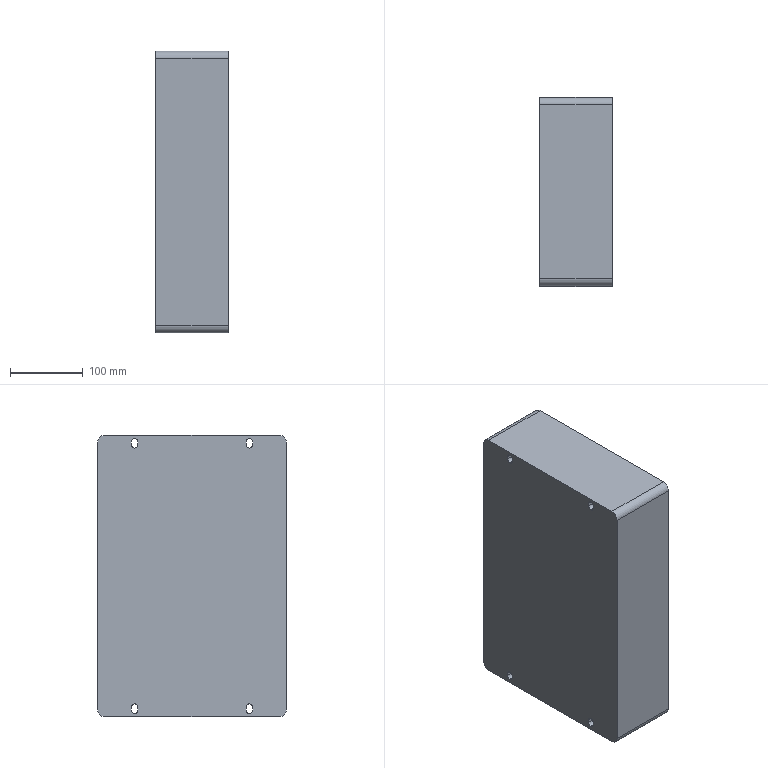Part | SolidWorks | 1 solid | 30 faces | box 100 x 260 x 388 mm | volume 10039569 mm3 | cylinder 16 | plane 14 | commonest cylinder face diameters 9 x12 20 x4
STEP:
#1=CARTESIAN_POINT('',(-50.,-79.,176.3));
#2=VERTEX_POINT('',#1);
#3=CARTESIAN_POINT('',(-50.,-74.5,180.8));
#4=VERTEX_POINT('',#3);
#5=CARTESIAN_POINT('',(-50.,-79.,180.8));
#6=DIRECTION('',(1.,0.,0.));
#7=DIRECTION('',(0.,0.,-1.));
#8=AXIS2_PLACEMENT_3D('',#5,#6,#7);
#9=CIRCLE('',#8,4.5);
#10=EDGE_CURVE('',#2,#4,#9,.T.);
#11=ORIENTED_EDGE('',*,*,#10,.F.);
#12=CARTESIAN_POINT('',(50.,-79.,176.3));
#13=VERTEX_POINT('',#12);
#14=CARTESIAN_POINT('',(-50.,-79.,176.3));
#15=DIRECTION('',(1.,0.,0.));
#16=VECTOR('',#15,1000.);
#17=LINE('',#14,#16);
#18=EDGE_CURVE('',#2,#13,#17,.T.);
#19=ORIENTED_EDGE('',*,*,#18,.T.);
#20=CARTESIAN_POINT('',(50.,-74.5,180.8));
#21=VERTEX_POINT('',#20);
#22=CARTESIAN_POINT('',(50.,-79.,180.8));
#23=DIRECTION('',(1.,0.,0.));
#24=DIRECTION('',(0.,0.,-1.));
#25=AXIS2_PLACEMENT_3D('',#22,#23,#24);
#26=CIRCLE('',#25,4.5);
#27=EDGE_CURVE('',#13,#21,#26,.T.);
#28=ORIENTED_EDGE('',*,*,#27,.T.);
#29=CARTESIAN_POINT('',(-50.,-74.5,180.8));
#30=DIRECTION('',(1.,0.,0.));
#31=VECTOR('',#30,1000.);
#32=LINE('',#29,#31);
#33=EDGE_CURVE('',#4,#21,#32,.T.);
#34=ORIENTED_EDGE('',*,*,#33,.F.);
#35=EDGE_LOOP('',(#11,#19,#28,#34));
#36=FACE_OUTER_BOUND('',#35,.T.);
#37=CARTESIAN_POINT('',(-50.,-79.,180.8));
#38=DIRECTION('',(1.,0.,0.));
#39=DIRECTION('',(0.,0.,-1.));
#40=AXIS2_PLACEMENT_3D('',#37,#38,#39);
#41=CYLINDRICAL_SURFACE('',#40,4.5);
#42=ADVANCED_FACE('',(#36),#41,.F.);
#43=CARTESIAN_POINT('',(-50.,-79.,-189.3));
#44=VERTEX_POINT('',#43);
#45=CARTESIAN_POINT('',(-50.,-74.5,-184.8));
#46=VERTEX_POINT('',#45);
#47=CARTESIAN_POINT('',(-50.,-79.,-184.8));
#48=DIRECTION('',(1.,0.,0.));
#49=DIRECTION('',(0.,0.,-1.));
#50=AXIS2_PLACEMENT_3D('',#47,#48,#49);
#51=CIRCLE('',#50,4.5);
#52=EDGE_CURVE('',#44,#46,#51,.T.);
#53=ORIENTED_EDGE('',*,*,#52,.F.);
#54=CARTESIAN_POINT('',(50.,-79.,-189.3));
#55=VERTEX_POINT('',#54);
#56=CARTESIAN_POINT('',(-50.,-79.,-189.3));
#57=DIRECTION('',(1.,0.,0.));
#58=VECTOR('',#57,1000.);
#59=LINE('',#56,#58);
#60=EDGE_CURVE('',#44,#55,#59,.T.);
#61=ORIENTED_EDGE('',*,*,#60,.T.);
#62=CARTESIAN_POINT('',(50.,-74.5,-184.8));
#63=VERTEX_POINT('',#62);
#64=CARTESIAN_POINT('',(50.,-79.,-184.8));
#65=DIRECTION('',(1.,0.,0.));
#66=DIRECTION('',(0.,0.,-1.));
#67=AXIS2_PLACEMENT_3D('',#64,#65,#66);
#68=CIRCLE('',#67,4.5);
#69=EDGE_CURVE('',#55,#63,#68,.T.);
#70=ORIENTED_EDGE('',*,*,#69,.T.);
#71=CARTESIAN_POINT('',(-50.,-74.5,-184.8));
#72=DIRECTION('',(1.,0.,0.));
#73=VECTOR('',#72,1000.);
#74=LINE('',#71,#73);
#75=EDGE_CURVE('',#46,#63,#74,.T.);
#76=ORIENTED_EDGE('',*,*,#75,.F.);
#77=EDGE_LOOP('',(#53,#61,#70,#76));
#78=FACE_OUTER_BOUND('',#77,.T.);
#79=CARTESIAN_POINT('',(-50.,-79.,-184.8));
#80=DIRECTION('',(1.,0.,0.));
#81=DIRECTION('',(0.,0.,-1.));
#82=AXIS2_PLACEMENT_3D('',#79,#80,#81);
#83=CYLINDRICAL_SURFACE('',#82,4.5);
#84=ADVANCED_FACE('',(#78),#83,.F.);
#85=CARTESIAN_POINT('',(-50.,79.,-189.3));
#86=VERTEX_POINT('',#85);
#87=CARTESIAN_POINT('',(-50.,83.5,-184.8));
#88=VERTEX_POINT('',#87);
#89=CARTESIAN_POINT('',(-50.,79.,-184.8));
#90=DIRECTION('',(1.,0.,0.));
#91=DIRECTION('',(0.,0.,-1.));
#92=AXIS2_PLACEMENT_3D('',#89,#90,#91);
#93=CIRCLE('',#92,4.5);
#94=EDGE_CURVE('',#86,#88,#93,.T.);
#95=ORIENTED_EDGE('',*,*,#94,.F.);
#96=CARTESIAN_POINT('',(50.,79.,-189.3));
#97=VERTEX_POINT('',#96);
#98=CARTESIAN_POINT('',(-50.,79.,-189.3));
#99=DIRECTION('',(1.,0.,0.));
#100=VECTOR('',#99,1000.);
#101=LINE('',#98,#100);
#102=EDGE_CURVE('',#86,#97,#101,.T.);
#103=ORIENTED_EDGE('',*,*,#102,.T.);
#104=CARTESIAN_POINT('',(50.,83.5,-184.8));
#105=VERTEX_POINT('',#104);
#106=CARTESIAN_POINT('',(50.,79.,-184.8));
#107=DIRECTION('',(1.,0.,0.));
#108=DIRECTION('',(0.,0.,-1.));
#109=AXIS2_PLACEMENT_3D('',#106,#107,#108);
#110=CIRCLE('',#109,4.5);
#111=EDGE_CURVE('',#97,#105,#110,.T.);
#112=ORIENTED_EDGE('',*,*,#111,.T.);
#113=CARTESIAN_POINT('',(-50.,83.5,-184.8));
#114=DIRECTION('',(1.,0.,0.));
#115=VECTOR('',#114,1000.);
#116=LINE('',#113,#115);
#117=EDGE_CURVE('',#88,#105,#116,.T.);
#118=ORIENTED_EDGE('',*,*,#117,.F.);
#119=EDGE_LOOP('',(#95,#103,#112,#118));
#120=FACE_OUTER_BOUND('',#119,.T.);
#121=CARTESIAN_POINT('',(-50.,79.,-184.8));
#122=DIRECTION('',(1.,0.,0.));
#123=DIRECTION('',(0.,0.,-1.));
#124=AXIS2_PLACEMENT_3D('',#121,#122,#123);
#125=CYLINDRICAL_SURFACE('',#124,4.5);
#126=ADVANCED_FACE('',(#120),#125,.F.);
#127=CARTESIAN_POINT('',(-50.,79.,176.3));
#128=VERTEX_POINT('',#127);
#129=CARTESIAN_POINT('',(-50.,83.5,180.8));
#130=VERTEX_POINT('',#129);
#131=CARTESIAN_POINT('',(-50.,79.,180.8));
#132=DIRECTION('',(1.,0.,0.));
#133=DIRECTION('',(0.,0.,-1.));
#134=AXIS2_PLACEMENT_3D('',#131,#132,#133);
#135=CIRCLE('',#134,4.5);
#136=EDGE_CURVE('',#128,#130,#135,.T.);
#137=ORIENTED_EDGE('',*,*,#136,.F.);
#138=CARTESIAN_POINT('',(50.,79.,176.3));
#139=VERTEX_POINT('',#138);
#140=CARTESIAN_POINT('',(-50.,79.,176.3));
#141=DIRECTION('',(1.,0.,0.));
#142=VECTOR('',#141,1000.);
#143=LINE('',#140,#142);
#144=EDGE_CURVE('',#128,#139,#143,.T.);
#145=ORIENTED_EDGE('',*,*,#144,.T.);
#146=CARTESIAN_POINT('',(50.,83.5,180.8));
#147=VERTEX_POINT('',#146);
#148=CARTESIAN_POINT('',(50.,79.,180.8));
#149=DIRECTION('',(1.,0.,0.));
#150=DIRECTION('',(0.,0.,-1.));
#151=AXIS2_PLACEMENT_3D('',#148,#149,#150);
#152=CIRCLE('',#151,4.5);
#153=EDGE_CURVE('',#139,#147,#152,.T.);
#154=ORIENTED_EDGE('',*,*,#153,.T.);
#155=CARTESIAN_POINT('',(-50.,83.5,180.8));
#156=DIRECTION('',(1.,0.,0.));
#157=VECTOR('',#156,1000.);
#158=LINE('',#155,#157);
#159=EDGE_CURVE('',#130,#147,#158,.T.);
#160=ORIENTED_EDGE('',*,*,#159,.F.);
#161=EDGE_LOOP('',(#137,#145,#154,#160));
#162=FACE_OUTER_BOUND('',#161,.T.);
#163=CARTESIAN_POINT('',(-50.,79.,180.8));
#164=DIRECTION('',(1.,0.,0.));
#165=DIRECTION('',(0.,0.,-1.));
#166=AXIS2_PLACEMENT_3D('',#163,#164,#165);
#167=CYLINDRICAL_SURFACE('',#166,4.5);
#168=ADVANCED_FACE('',(#162),#167,.F.);
#169=CARTESIAN_POINT('',(-50.,120.,194.));
#170=VERTEX_POINT('',#169);
#171=CARTESIAN_POINT('',(-50.,-120.,194.));
#172=VERTEX_POINT('',#171);
#173=CARTESIAN_POINT('',(-50.,-130.,194.));
#174=DIRECTION('',(0.,-1.,0.));
#175=VECTOR('',#174,1000.);
#176=LINE('',#173,#175);
#177=EDGE_CURVE('',#170,#172,#176,.T.);
#178=ORIENTED_EDGE('',*,*,#177,.T.);
#179=CARTESIAN_POINT('',(50.,-120.,194.));
#180=VERTEX_POINT('',#179);
#181=CARTESIAN_POINT('',(50.,-120.,194.));
#182=DIRECTION('',(1.,0.,0.));
#183=VECTOR('',#182,1000.);
#184=LINE('',#181,#183);
#185=EDGE_CURVE('',#172,#180,#184,.T.);
#186=ORIENTED_EDGE('',*,*,#185,.T.);
#187=CARTESIAN_POINT('',(50.,120.,194.));
#188=VERTEX_POINT('',#187);
#189=CARTESIAN_POINT('',(50.,-130.,194.));
#190=DIRECTION('',(0.,-1.,0.));
#191=VECTOR('',#190,1000.);
#192=LINE('',#189,#191);
#193=EDGE_CURVE('',#188,#180,#192,.T.);
#194=ORIENTED_EDGE('',*,*,#193,.F.);
#195=CARTESIAN_POINT('',(50.,120.,194.));
#196=DIRECTION('',(-1.,0.,0.));
#197=VECTOR('',#196,1000.);
#198=LINE('',#195,#197);
#199=EDGE_CURVE('',#188,#170,#198,.T.);
#200=ORIENTED_EDGE('',*,*,#199,.T.);
#201=EDGE_LOOP('',(#178,#186,#194,#200));
#202=FACE_OUTER_BOUND('',#201,.T.);
#203=CARTESIAN_POINT('',(50.,-130.,194.));
#204=DIRECTION('',(0.,0.,-1.));
#205=DIRECTION('',(-1.,0.,0.));
#206=AXIS2_PLACEMENT_3D('',#203,#204,#205);
#207=PLANE('',#206);
#208=ADVANCED_FACE('',(#202),#207,.F.);
#209=CARTESIAN_POINT('',(-50.,-130.,184.));
#210=VERTEX_POINT('',#209);
#211=CARTESIAN_POINT('',(-50.,-130.,-184.));
#212=VERTEX_POINT('',#211);
#213=CARTESIAN_POINT('',(-50.,-130.,-194.));
#214=DIRECTION('',(0.,0.,-1.));
#215=VECTOR('',#214,1000.);
#216=LINE('',#213,#215);
#217=EDGE_CURVE('',#210,#212,#216,.T.);
#218=ORIENTED_EDGE('',*,*,#217,.T.);
#219=CARTESIAN_POINT('',(50.,-130.,-184.));
#220=VERTEX_POINT('',#219);
#221=CARTESIAN_POINT('',(50.,-130.,-184.));
#222=DIRECTION('',(1.,0.,0.));
#223=VECTOR('',#222,1000.);
#224=LINE('',#221,#223);
#225=EDGE_CURVE('',#212,#220,#224,.T.);
#226=ORIENTED_EDGE('',*,*,#225,.T.);
#227=CARTESIAN_POINT('',(50.,-130.,184.));
#228=VERTEX_POINT('',#227);
#229=CARTESIAN_POINT('',(50.,-130.,-194.));
#230=DIRECTION('',(0.,0.,-1.));
#231=VECTOR('',#230,1000.);
#232=LINE('',#229,#231);
#233=EDGE_CURVE('',#228,#220,#232,.T.);
#234=ORIENTED_EDGE('',*,*,#233,.F.);
#235=CARTESIAN_POINT('',(50.,-130.,184.));
#236=DIRECTION('',(-1.,0.,0.));
#237=VECTOR('',#236,1000.);
#238=LINE('',#235,#237);
#239=EDGE_CURVE('',#228,#210,#238,.T.);
#240=ORIENTED_EDGE('',*,*,#239,.T.);
#241=EDGE_LOOP('',(#218,#226,#234,#240));
#242=FACE_OUTER_BOUND('',#241,.T.);
#243=CARTESIAN_POINT('',(50.,-130.,-194.));
#244=DIRECTION('',(0.,1.,0.));
#245=DIRECTION('',(0.,0.,1.));
#246=AXIS2_PLACEMENT_3D('',#243,#244,#245);
#247=PLANE('',#246);
#248=ADVANCED_FACE('',(#242),#247,.F.);
#249=CARTESIAN_POINT('',(-50.,-120.,-194.));
#250=VERTEX_POINT('',#249);
#251=CARTESIAN_POINT('',(-50.,120.,-194.));
#252=VERTEX_POINT('',#251);
#253=CARTESIAN_POINT('',(-50.,-130.,-194.));
#254=DIRECTION('',(0.,1.,0.));
#255=VECTOR('',#254,1000.);
#256=LINE('',#253,#255);
#257=EDGE_CURVE('',#250,#252,#256,.T.);
#258=ORIENTED_EDGE('',*,*,#257,.T.);
#259=CARTESIAN_POINT('',(50.,120.,-194.));
#260=VERTEX_POINT('',#259);
#261=CARTESIAN_POINT('',(50.,120.,-194.));
#262=DIRECTION('',(1.,0.,0.));
#263=VECTOR('',#262,1000.);
#264=LINE('',#261,#263);
#265=EDGE_CURVE('',#252,#260,#264,.T.);
#266=ORIENTED_EDGE('',*,*,#265,.T.);
#267=CARTESIAN_POINT('',(50.,-120.,-194.));
#268=VERTEX_POINT('',#267);
#269=CARTESIAN_POINT('',(50.,-130.,-194.));
#270=DIRECTION('',(0.,1.,0.));
#271=VECTOR('',#270,1000.);
#272=LINE('',#269,#271);
#273=EDGE_CURVE('',#268,#260,#272,.T.);
#274=ORIENTED_EDGE('',*,*,#273,.F.);
#275=CARTESIAN_POINT('',(50.,-120.,-194.));
#276=DIRECTION('',(-1.,0.,0.));
#277=VECTOR('',#276,1000.);
#278=LINE('',#275,#277);
#279=EDGE_CURVE('',#268,#250,#278,.T.);
#280=ORIENTED_EDGE('',*,*,#279,.T.);
#281=EDGE_LOOP('',(#258,#266,#274,#280));
#282=FACE_OUTER_BOUND('',#281,.T.);
#283=CARTESIAN_POINT('',(50.,-130.,-194.));
#284=DIRECTION('',(0.,0.,1.));
#285=DIRECTION('',(1.,0.,0.));
#286=AXIS2_PLACEMENT_3D('',#283,#284,#285);
#287=PLANE('',#286);
#288=ADVANCED_FACE('',(#282),#287,.F.);
#289=CARTESIAN_POINT('',(50.,130.,-184.));
#290=VERTEX_POINT('',#289);
#291=CARTESIAN_POINT('',(50.,130.,184.));
#292=VERTEX_POINT('',#291);
#293=CARTESIAN_POINT('',(50.,130.,-194.));
#294=DIRECTION('',(0.,0.,1.));
#295=VECTOR('',#294,1000.);
#296=LINE('',#293,#295);
#297=EDGE_CURVE('',#290,#292,#296,.T.);
#298=ORIENTED_EDGE('',*,*,#297,.F.);
#299=CARTESIAN_POINT('',(-50.,130.,-184.));
#300=VERTEX_POINT('',#299);
#301=CARTESIAN_POINT('',(50.,130.,-184.));
#302=DIRECTION('',(-1.,0.,0.));
#303=VECTOR('',#302,1000.);
#304=LINE('',#301,#303);
#305=EDGE_CURVE('',#290,#300,#304,.T.);
#306=ORIENTED_EDGE('',*,*,#305,.T.);
#307=CARTESIAN_POINT('',(-50.,130.,184.));
#308=VERTEX_POINT('',#307);
#309=CARTESIAN_POINT('',(-50.,130.,-194.));
#310=DIRECTION('',(0.,0.,1.));
#311=VECTOR('',#310,1000.);
#312=LINE('',#309,#311);
#313=EDGE_CURVE('',#300,#308,#312,.T.);
#314=ORIENTED_EDGE('',*,*,#313,.T.);
#315=CARTESIAN_POINT('',(50.,130.,184.));
#316=DIRECTION('',(1.,0.,0.));
#317=VECTOR('',#316,1000.);
#318=LINE('',#315,#317);
#319=EDGE_CURVE('',#308,#292,#318,.T.);
#320=ORIENTED_EDGE('',*,*,#319,.T.);
#321=EDGE_LOOP('',(#298,#306,#314,#320));
#322=FACE_OUTER_BOUND('',#321,.T.);
#323=CARTESIAN_POINT('',(50.,130.,-194.));
#324=DIRECTION('',(0.,-1.,0.));
#325=DIRECTION('',(0.,0.,-1.));
#326=AXIS2_PLACEMENT_3D('',#323,#324,#325);
#327=PLANE('',#326);
#328=ADVANCED_FACE('',(#322),#327,.F.);
#329=CARTESIAN_POINT('',(50.,-74.5,184.8));
#330=VERTEX_POINT('',#329);
#331=CARTESIAN_POINT('',(50.,-83.5,184.8));
#332=VERTEX_POINT('',#331);
#333=CARTESIAN_POINT('',(50.,-79.,184.8));
#334=DIRECTION('',(1.,0.,0.));
#335=DIRECTION('',(0.,0.,-1.));
#336=AXIS2_PLACEMENT_3D('',#333,#334,#335);
#337=CIRCLE('',#336,4.5);
#338=EDGE_CURVE('',#330,#332,#337,.T.);
#339=ORIENTED_EDGE('',*,*,#338,.F.);
#340=CARTESIAN_POINT('',(50.,-74.5,184.8));
#341=DIRECTION('',(0.,0.,1.));
#342=VECTOR('',#341,1000.);
#343=LINE('',#340,#342);
#344=EDGE_CURVE('',#21,#330,#343,.T.);
#345=ORIENTED_EDGE('',*,*,#344,.F.);
#346=ORIENTED_EDGE('',*,*,#27,.F.);
#347=CARTESIAN_POINT('',(50.,-83.5,180.8));
#348=VERTEX_POINT('',#347);
#349=CARTESIAN_POINT('',(50.,-79.,180.8));
#350=DIRECTION('',(1.,0.,0.));
#351=DIRECTION('',(0.,0.,-1.));
#352=AXIS2_PLACEMENT_3D('',#349,#350,#351);
#353=CIRCLE('',#352,4.5);
#354=EDGE_CURVE('',#348,#13,#353,.T.);
#355=ORIENTED_EDGE('',*,*,#354,.F.);
#356=CARTESIAN_POINT('',(50.,-83.5,184.8));
#357=DIRECTION('',(0.,0.,-1.));
#358=VECTOR('',#357,1000.);
#359=LINE('',#356,#358);
#360=EDGE_CURVE('',#332,#348,#359,.T.);
#361=ORIENTED_EDGE('',*,*,#360,.F.);
#362=EDGE_LOOP('',(#339,#345,#346,#355,#361));
#363=FACE_BOUND('',#362,.T.);
#364=CARTESIAN_POINT('',(50.,-74.5,-180.8));
#365=VERTEX_POINT('',#364);
#366=CARTESIAN_POINT('',(50.,-83.5,-180.8));
#367=VERTEX_POINT('',#366);
#368=CARTESIAN_POINT('',(50.,-79.,-180.8));
#369=DIRECTION('',(1.,0.,0.));
#370=DIRECTION('',(0.,0.,-1.));
#371=AXIS2_PLACEMENT_3D('',#368,#369,#370);
#372=CIRCLE('',#371,4.5);
#373=EDGE_CURVE('',#365,#367,#372,.T.);
#374=ORIENTED_EDGE('',*,*,#373,.F.);
#375=CARTESIAN_POINT('',(50.,-74.5,-180.8));
#376=DIRECTION('',(0.,0.,1.));
#377=VECTOR('',#376,1000.);
#378=LINE('',#375,#377);
#379=EDGE_CURVE('',#63,#365,#378,.T.);
#380=ORIENTED_EDGE('',*,*,#379,.F.);
#381=ORIENTED_EDGE('',*,*,#69,.F.);
#382=CARTESIAN_POINT('',(50.,-83.5,-184.8));
#383=VERTEX_POINT('',#382);
#384=CARTESIAN_POINT('',(50.,-79.,-184.8));
#385=DIRECTION('',(1.,0.,0.));
#386=DIRECTION('',(0.,0.,-1.));
#387=AXIS2_PLACEMENT_3D('',#384,#385,#386);
#388=CIRCLE('',#387,4.5);
#389=EDGE_CURVE('',#383,#55,#388,.T.);
#390=ORIENTED_EDGE('',*,*,#389,.F.);
#391=CARTESIAN_POINT('',(50.,-83.5,-180.8));
#392=DIRECTION('',(0.,0.,-1.));
#393=VECTOR('',#392,1000.);
#394=LINE('',#391,#393);
#395=EDGE_CURVE('',#367,#383,#394,.T.);
#396=ORIENTED_EDGE('',*,*,#395,.F.);
#397=EDGE_LOOP('',(#374,#380,#381,#390,#396));
#398=FACE_BOUND('',#397,.T.);
#399=CARTESIAN_POINT('',(50.,83.5,-180.8));
#400=VERTEX_POINT('',#399);
#401=CARTESIAN_POINT('',(50.,74.5,-180.8));
#402=VERTEX_POINT('',#401);
#403=CARTESIAN_POINT('',(50.,79.,-180.8));
#404=DIRECTION('',(1.,0.,0.));
#405=DIRECTION('',(0.,0.,-1.));
#406=AXIS2_PLACEMENT_3D('',#403,#404,#405);
#407=CIRCLE('',#406,4.5);
#408=EDGE_CURVE('',#400,#402,#407,.T.);
#409=ORIENTED_EDGE('',*,*,#408,.F.);
#410=CARTESIAN_POINT('',(50.,83.5,-180.8));
#411=DIRECTION('',(0.,0.,1.));
#412=VECTOR('',#411,1000.);
#413=LINE('',#410,#412);
#414=EDGE_CURVE('',#105,#400,#413,.T.);
#415=ORIENTED_EDGE('',*,*,#414,.F.);
#416=ORIENTED_EDGE('',*,*,#111,.F.);
#417=CARTESIAN_POINT('',(50.,74.5,-184.8));
#418=VERTEX_POINT('',#417);
#419=CARTESIAN_POINT('',(50.,79.,-184.8));
#420=DIRECTION('',(1.,0.,0.));
#421=DIRECTION('',(0.,0.,-1.));
#422=AXIS2_PLACEMENT_3D('',#419,#420,#421);
#423=CIRCLE('',#422,4.5);
#424=EDGE_CURVE('',#418,#97,#423,.T.);
#425=ORIENTED_EDGE('',*,*,#424,.F.);
#426=CARTESIAN_POINT('',(50.,74.5,-180.8));
#427=DIRECTION('',(0.,0.,-1.));
#428=VECTOR('',#427,1000.);
#429=LINE('',#426,#428);
#430=EDGE_CURVE('',#402,#418,#429,.T.);
#431=ORIENTED_EDGE('',*,*,#430,.F.);
#432=EDGE_LOOP('',(#409,#415,#416,#425,#431));
#433=FACE_BOUND('',#432,.T.);
#434=CARTESIAN_POINT('',(50.,83.5,184.8));
#435=VERTEX_POINT('',#434);
#436=CARTESIAN_POINT('',(50.,74.5,184.8));
#437=VERTEX_POINT('',#436);
#438=CARTESIAN_POINT('',(50.,79.,184.8));
#439=DIRECTION('',(1.,0.,0.));
#440=DIRECTION('',(0.,0.,-1.));
#441=AXIS2_PLACEMENT_3D('',#438,#439,#440);
#442=CIRCLE('',#441,4.5);
#443=EDGE_CURVE('',#435,#437,#442,.T.);
#444=ORIENTED_EDGE('',*,*,#443,.F.);
#445=CARTESIAN_POINT('',(50.,83.5,184.8));
#446=DIRECTION('',(0.,0.,1.));
#447=VECTOR('',#446,1000.);
#448=LINE('',#445,#447);
#449=EDGE_CURVE('',#147,#435,#448,.T.);
#450=ORIENTED_EDGE('',*,*,#449,.F.);
#451=ORIENTED_EDGE('',*,*,#153,.F.);
#452=CARTESIAN_POINT('',(50.,74.5,180.8));
#453=VERTEX_POINT('',#452);
#454=CARTESIAN_POINT('',(50.,79.,180.8));
#455=DIRECTION('',(1.,0.,0.));
#456=DIRECTION('',(0.,0.,-1.));
#457=AXIS2_PLACEMENT_3D('',#454,#455,#456);
#458=CIRCLE('',#457,4.5);
#459=EDGE_CURVE('',#453,#139,#458,.T.);
#460=ORIENTED_EDGE('',*,*,#459,.F.);
#461=CARTESIAN_POINT('',(50.,74.5,184.8));
#462=DIRECTION('',(0.,0.,-1.));
#463=VECTOR('',#462,1000.);
#464=LINE('',#461,#463);
#465=EDGE_CURVE('',#437,#453,#464,.T.);
#466=ORIENTED_EDGE('',*,*,#465,.F.);
#467=EDGE_LOOP('',(#444,#450,#451,#460,#466));
#468=FACE_BOUND('',#467,.T.);
#469=ORIENTED_EDGE('',*,*,#273,.T.);
#470=CARTESIAN_POINT('',(50.,120.,-184.));
#471=DIRECTION('',(1.,0.,0.));
#472=DIRECTION('',(0.,0.,-1.));
#473=AXIS2_PLACEMENT_3D('',#470,#471,#472);
#474=CIRCLE('',#473,10.);
#475=EDGE_CURVE('',#260,#290,#474,.T.);
#476=ORIENTED_EDGE('',*,*,#475,.T.);
#477=ORIENTED_EDGE('',*,*,#297,.T.);
#478=CARTESIAN_POINT('',(50.,120.,184.));
#479=DIRECTION('',(1.,0.,0.));
#480=DIRECTION('',(0.,0.,-1.));
#481=AXIS2_PLACEMENT_3D('',#478,#479,#480);
#482=CIRCLE('',#481,10.);
#483=EDGE_CURVE('',#292,#188,#482,.T.);
#484=ORIENTED_EDGE('',*,*,#483,.T.);
#485=ORIENTED_EDGE('',*,*,#193,.T.);
#486=CARTESIAN_POINT('',(50.,-120.,184.));
#487=DIRECTION('',(1.,0.,0.));
#488=DIRECTION('',(0.,0.,-1.));
#489=AXIS2_PLACEMENT_3D('',#486,#487,#488);
#490=CIRCLE('',#489,10.);
#491=EDGE_CURVE('',#180,#228,#490,.T.);
#492=ORIENTED_EDGE('',*,*,#491,.T.);
#493=ORIENTED_EDGE('',*,*,#233,.T.);
#494=CARTESIAN_POINT('',(50.,-120.,-184.));
#495=DIRECTION('',(1.,0.,0.));
#496=DIRECTION('',(0.,0.,-1.));
#497=AXIS2_PLACEMENT_3D('',#494,#495,#496);
#498=CIRCLE('',#497,10.);
#499=EDGE_CURVE('',#220,#268,#498,.T.);
#500=ORIENTED_EDGE('',*,*,#499,.T.);
#501=EDGE_LOOP('',(#469,#476,#477,#484,#485,#492,#493,#500));
#502=FACE_OUTER_BOUND('',#501,.T.);
#503=CARTESIAN_POINT('',(50.,0.,0.));
#504=DIRECTION('',(1.,0.,0.));
#505=DIRECTION('',(0.,0.,-1.));
#506=AXIS2_PLACEMENT_3D('',#503,#504,#505);
#507=PLANE('',#506);
#508=ADVANCED_FACE('',(#363,#398,#433,#468,#502),#507,.T.);
#509=CARTESIAN_POINT('',(-50.,-74.5,184.8));
#510=VERTEX_POINT('',#509);
#511=CARTESIAN_POINT('',(-50.,-74.5,184.8));
#512=DIRECTION('',(0.,0.,1.));
#513=VECTOR('',#512,1000.);
#514=LINE('',#511,#513);
#515=EDGE_CURVE('',#4,#510,#514,.T.);
#516=ORIENTED_EDGE('',*,*,#515,.T.);
#517=CARTESIAN_POINT('',(-50.,-83.5,184.8));
#518=VERTEX_POINT('',#517);
#519=CARTESIAN_POINT('',(-50.,-79.,184.8));
#520=DIRECTION('',(1.,0.,0.));
#521=DIRECTION('',(0.,0.,-1.));
#522=AXIS2_PLACEMENT_3D('',#519,#520,#521);
#523=CIRCLE('',#522,4.5);
#524=EDGE_CURVE('',#510,#518,#523,.T.);
#525=ORIENTED_EDGE('',*,*,#524,.T.);
#526=CARTESIAN_POINT('',(-50.,-83.5,180.8));
#527=VERTEX_POINT('',#526);
#528=CARTESIAN_POINT('',(-50.,-83.5,184.8));
#529=DIRECTION('',(0.,0.,-1.));
#530=VECTOR('',#529,1000.);
#531=LINE('',#528,#530);
#532=EDGE_CURVE('',#518,#527,#531,.T.);
#533=ORIENTED_EDGE('',*,*,#532,.T.);
#534=CARTESIAN_POINT('',(-50.,-79.,180.8));
#535=DIRECTION('',(1.,0.,0.));
#536=DIRECTION('',(0.,0.,-1.));
#537=AXIS2_PLACEMENT_3D('',#534,#535,#536);
#538=CIRCLE('',#537,4.5);
#539=EDGE_CURVE('',#527,#2,#538,.T.);
#540=ORIENTED_EDGE('',*,*,#539,.T.);
#541=ORIENTED_EDGE('',*,*,#10,.T.);
#542=EDGE_LOOP('',(#516,#525,#533,#540,#541));
#543=FACE_BOUND('',#542,.T.);
#544=CARTESIAN_POINT('',(-50.,-74.5,-180.8));
#545=VERTEX_POINT('',#544);
#546=CARTESIAN_POINT('',(-50.,-74.5,-180.8));
#547=DIRECTION('',(0.,0.,1.));
#548=VECTOR('',#547,1000.);
#549=LINE('',#546,#548);
#550=EDGE_CURVE('',#46,#545,#549,.T.);
#551=ORIENTED_EDGE('',*,*,#550,.T.);
#552=CARTESIAN_POINT('',(-50.,-83.5,-180.8));
#553=VERTEX_POINT('',#552);
#554=CARTESIAN_POINT('',(-50.,-79.,-180.8));
#555=DIRECTION('',(1.,0.,0.));
#556=DIRECTION('',(0.,0.,-1.));
#557=AXIS2_PLACEMENT_3D('',#554,#555,#556);
#558=CIRCLE('',#557,4.5);
#559=EDGE_CURVE('',#545,#553,#558,.T.);
#560=ORIENTED_EDGE('',*,*,#559,.T.);
#561=CARTESIAN_POINT('',(-50.,-83.5,-184.8));
#562=VERTEX_POINT('',#561);
#563=CARTESIAN_POINT('',(-50.,-83.5,-180.8));
#564=DIRECTION('',(0.,0.,-1.));
#565=VECTOR('',#564,1000.);
#566=LINE('',#563,#565);
#567=EDGE_CURVE('',#553,#562,#566,.T.);
#568=ORIENTED_EDGE('',*,*,#567,.T.);
#569=CARTESIAN_POINT('',(-50.,-79.,-184.8));
#570=DIRECTION('',(1.,0.,0.));
#571=DIRECTION('',(0.,0.,-1.));
#572=AXIS2_PLACEMENT_3D('',#569,#570,#571);
#573=CIRCLE('',#572,4.5);
#574=EDGE_CURVE('',#562,#44,#573,.T.);
#575=ORIENTED_EDGE('',*,*,#574,.T.);
#576=ORIENTED_EDGE('',*,*,#52,.T.);
#577=EDGE_LOOP('',(#551,#560,#568,#575,#576));
#578=FACE_BOUND('',#577,.T.);
#579=CARTESIAN_POINT('',(-50.,83.5,-180.8));
#580=VERTEX_POINT('',#579);
#581=CARTESIAN_POINT('',(-50.,83.5,-180.8));
#582=DIRECTION('',(0.,0.,1.));
#583=VECTOR('',#582,1000.);
#584=LINE('',#581,#583);
#585=EDGE_CURVE('',#88,#580,#584,.T.);
#586=ORIENTED_EDGE('',*,*,#585,.T.);
#587=CARTESIAN_POINT('',(-50.,74.5,-180.8));
#588=VERTEX_POINT('',#587);
#589=CARTESIAN_POINT('',(-50.,79.,-180.8));
#590=DIRECTION('',(1.,0.,0.));
#591=DIRECTION('',(0.,0.,-1.));
#592=AXIS2_PLACEMENT_3D('',#589,#590,#591);
#593=CIRCLE('',#592,4.5);
#594=EDGE_CURVE('',#580,#588,#593,.T.);
#595=ORIENTED_EDGE('',*,*,#594,.T.);
#596=CARTESIAN_POINT('',(-50.,74.5,-184.8));
#597=VERTEX_POINT('',#596);
#598=CARTESIAN_POINT('',(-50.,74.5,-180.8));
#599=DIRECTION('',(0.,0.,-1.));
#600=VECTOR('',#599,1000.);
#601=LINE('',#598,#600);
#602=EDGE_CURVE('',#588,#597,#601,.T.);
#603=ORIENTED_EDGE('',*,*,#602,.T.);
#604=CARTESIAN_POINT('',(-50.,79.,-184.8));
#605=DIRECTION('',(1.,0.,0.));
#606=DIRECTION('',(0.,0.,-1.));
#607=AXIS2_PLACEMENT_3D('',#604,#605,#606);
#608=CIRCLE('',#607,4.5);
#609=EDGE_CURVE('',#597,#86,#608,.T.);
#610=ORIENTED_EDGE('',*,*,#609,.T.);
#611=ORIENTED_EDGE('',*,*,#94,.T.);
#612=EDGE_LOOP('',(#586,#595,#603,#610,#611));
#613=FACE_BOUND('',#612,.T.);
#614=CARTESIAN_POINT('',(-50.,83.5,184.8));
#615=VERTEX_POINT('',#614);
#616=CARTESIAN_POINT('',(-50.,83.5,184.8));
#617=DIRECTION('',(0.,0.,1.));
#618=VECTOR('',#617,1000.);
#619=LINE('',#616,#618);
#620=EDGE_CURVE('',#130,#615,#619,.T.);
#621=ORIENTED_EDGE('',*,*,#620,.T.);
#622=CARTESIAN_POINT('',(-50.,74.5,184.8));
#623=VERTEX_POINT('',#622);
#624=CARTESIAN_POINT('',(-50.,79.,184.8));
#625=DIRECTION('',(1.,0.,0.));
#626=DIRECTION('',(0.,0.,-1.));
#627=AXIS2_PLACEMENT_3D('',#624,#625,#626);
#628=CIRCLE('',#627,4.5);
#629=EDGE_CURVE('',#615,#623,#628,.T.);
#630=ORIENTED_EDGE('',*,*,#629,.T.);
#631=CARTESIAN_POINT('',(-50.,74.5,180.8));
#632=VERTEX_POINT('',#631);
#633=CARTESIAN_POINT('',(-50.,74.5,184.8));
#634=DIRECTION('',(0.,0.,-1.));
#635=VECTOR('',#634,1000.);
#636=LINE('',#633,#635);
#637=EDGE_CURVE('',#623,#632,#636,.T.);
#638=ORIENTED_EDGE('',*,*,#637,.T.);
#639=CARTESIAN_POINT('',(-50.,79.,180.8));
#640=DIRECTION('',(1.,0.,0.));
#641=DIRECTION('',(0.,0.,-1.));
#642=AXIS2_PLACEMENT_3D('',#639,#640,#641);
#643=CIRCLE('',#642,4.5);
#644=EDGE_CURVE('',#632,#128,#643,.T.);
#645=ORIENTED_EDGE('',*,*,#644,.T.);
#646=ORIENTED_EDGE('',*,*,#136,.T.);
#647=EDGE_LOOP('',(#621,#630,#638,#645,#646));
#648=FACE_BOUND('',#647,.T.);
#649=ORIENTED_EDGE('',*,*,#313,.F.);
#650=CARTESIAN_POINT('',(-50.,120.,-184.));
#651=DIRECTION('',(-1.,0.,0.));
#652=DIRECTION('',(0.,0.,-1.));
#653=AXIS2_PLACEMENT_3D('',#650,#651,#652);
#654=CIRCLE('',#653,10.);
#655=EDGE_CURVE('',#300,#252,#654,.T.);
#656=ORIENTED_EDGE('',*,*,#655,.T.);
#657=ORIENTED_EDGE('',*,*,#257,.F.);
#658=CARTESIAN_POINT('',(-50.,-120.,-184.));
#659=DIRECTION('',(-1.,0.,0.));
#660=DIRECTION('',(0.,0.,-1.));
#661=AXIS2_PLACEMENT_3D('',#658,#659,#660);
#662=CIRCLE('',#661,10.);
#663=EDGE_CURVE('',#250,#212,#662,.T.);
#664=ORIENTED_EDGE('',*,*,#663,.T.);
#665=ORIENTED_EDGE('',*,*,#217,.F.);
#666=CARTESIAN_POINT('',(-50.,-120.,184.));
#667=DIRECTION('',(-1.,0.,0.));
#668=DIRECTION('',(0.,0.,-1.));
#669=AXIS2_PLACEMENT_3D('',#666,#667,#668);
#670=CIRCLE('',#669,10.);
#671=EDGE_CURVE('',#210,#172,#670,.T.);
#672=ORIENTED_EDGE('',*,*,#671,.T.);
#673=ORIENTED_EDGE('',*,*,#177,.F.);
#674=CARTESIAN_POINT('',(-50.,120.,184.));
#675=DIRECTION('',(-1.,0.,0.));
#676=DIRECTION('',(0.,0.,-1.));
#677=AXIS2_PLACEMENT_3D('',#674,#675,#676);
#678=CIRCLE('',#677,10.);
#679=EDGE_CURVE('',#170,#308,#678,.T.);
#680=ORIENTED_EDGE('',*,*,#679,.T.);
#681=EDGE_LOOP('',(#649,#656,#657,#664,#665,#672,#673,#680));
#682=FACE_OUTER_BOUND('',#681,.T.);
#683=CARTESIAN_POINT('',(-50.,0.,0.));
#684=DIRECTION('',(1.,0.,0.));
#685=DIRECTION('',(0.,0.,-1.));
#686=AXIS2_PLACEMENT_3D('',#683,#684,#685);
#687=PLANE('',#686);
#688=ADVANCED_FACE('',(#543,#578,#613,#648,#682),#687,.F.);
#689=ORIENTED_EDGE('',*,*,#443,.T.);
#690=CARTESIAN_POINT('',(-50.,74.5,184.8));
#691=DIRECTION('',(1.,0.,0.));
#692=VECTOR('',#691,1000.);
#693=LINE('',#690,#692);
#694=EDGE_CURVE('',#623,#437,#693,.T.);
#695=ORIENTED_EDGE('',*,*,#694,.F.);
#696=ORIENTED_EDGE('',*,*,#629,.F.);
#697=CARTESIAN_POINT('',(-50.,83.5,184.8));
#698=DIRECTION('',(1.,0.,0.));
#699=VECTOR('',#698,1000.);
#700=LINE('',#697,#699);
#701=EDGE_CURVE('',#615,#435,#700,.T.);
#702=ORIENTED_EDGE('',*,*,#701,.T.);
#703=EDGE_LOOP('',(#689,#695,#696,#702));
#704=FACE_OUTER_BOUND('',#703,.T.);
#705=CARTESIAN_POINT('',(-50.,79.,184.8));
#706=DIRECTION('',(1.,0.,0.));
#707=DIRECTION('',(0.,0.,-1.));
#708=AXIS2_PLACEMENT_3D('',#705,#706,#707);
#709=CYLINDRICAL_SURFACE('',#708,4.5);
#710=ADVANCED_FACE('',(#704),#709,.F.);
#711=ORIENTED_EDGE('',*,*,#449,.T.);
#712=ORIENTED_EDGE('',*,*,#701,.F.);
#713=ORIENTED_EDGE('',*,*,#620,.F.);
#714=ORIENTED_EDGE('',*,*,#159,.T.);
#715=EDGE_LOOP('',(#711,#712,#713,#714));
#716=FACE_OUTER_BOUND('',#715,.T.);
#717=CARTESIAN_POINT('',(-50.,83.5,184.8));
#718=DIRECTION('',(0.,1.,0.));
#719=DIRECTION('',(0.,0.,1.));
#720=AXIS2_PLACEMENT_3D('',#717,#718,#719);
#721=PLANE('',#720);
#722=ADVANCED_FACE('',(#716),#721,.F.);
#723=ORIENTED_EDGE('',*,*,#144,.F.);
#724=ORIENTED_EDGE('',*,*,#644,.F.);
#725=CARTESIAN_POINT('',(-50.,74.5,180.8));
#726=DIRECTION('',(1.,0.,0.));
#727=VECTOR('',#726,1000.);
#728=LINE('',#725,#727);
#729=EDGE_CURVE('',#632,#453,#728,.T.);
#730=ORIENTED_EDGE('',*,*,#729,.T.);
#731=ORIENTED_EDGE('',*,*,#459,.T.);
#732=EDGE_LOOP('',(#723,#724,#730,#731));
#733=FACE_OUTER_BOUND('',#732,.T.);
#734=CARTESIAN_POINT('',(-50.,79.,180.8));
#735=DIRECTION('',(1.,0.,0.));
#736=DIRECTION('',(0.,0.,-1.));
#737=AXIS2_PLACEMENT_3D('',#734,#735,#736);
#738=CYLINDRICAL_SURFACE('',#737,4.5);
#739=ADVANCED_FACE('',(#733),#738,.F.);
#740=ORIENTED_EDGE('',*,*,#465,.T.);
#741=ORIENTED_EDGE('',*,*,#729,.F.);
#742=ORIENTED_EDGE('',*,*,#637,.F.);
#743=ORIENTED_EDGE('',*,*,#694,.T.);
#744=EDGE_LOOP('',(#740,#741,#742,#743));
#745=FACE_OUTER_BOUND('',#744,.T.);
#746=CARTESIAN_POINT('',(-50.,74.5,184.8));
#747=DIRECTION('',(0.,-1.,0.));
#748=DIRECTION('',(0.,0.,-1.));
#749=AXIS2_PLACEMENT_3D('',#746,#747,#748);
#750=PLANE('',#749);
#751=ADVANCED_FACE('',(#745),#750,.F.);
#752=ORIENTED_EDGE('',*,*,#408,.T.);
#753=CARTESIAN_POINT('',(-50.,74.5,-180.8));
#754=DIRECTION('',(1.,0.,0.));
#755=VECTOR('',#754,1000.);
#756=LINE('',#753,#755);
#757=EDGE_CURVE('',#588,#402,#756,.T.);
#758=ORIENTED_EDGE('',*,*,#757,.F.);
#759=ORIENTED_EDGE('',*,*,#594,.F.);
#760=CARTESIAN_POINT('',(-50.,83.5,-180.8));
#761=DIRECTION('',(1.,0.,0.));
#762=VECTOR('',#761,1000.);
#763=LINE('',#760,#762);
#764=EDGE_CURVE('',#580,#400,#763,.T.);
#765=ORIENTED_EDGE('',*,*,#764,.T.);
#766=EDGE_LOOP('',(#752,#758,#759,#765));
#767=FACE_OUTER_BOUND('',#766,.T.);
#768=CARTESIAN_POINT('',(-50.,79.,-180.8));
#769=DIRECTION('',(1.,0.,0.));
#770=DIRECTION('',(0.,0.,-1.));
#771=AXIS2_PLACEMENT_3D('',#768,#769,#770);
#772=CYLINDRICAL_SURFACE('',#771,4.5);
#773=ADVANCED_FACE('',(#767),#772,.F.);
#774=ORIENTED_EDGE('',*,*,#414,.T.);
#775=ORIENTED_EDGE('',*,*,#764,.F.);
#776=ORIENTED_EDGE('',*,*,#585,.F.);
#777=ORIENTED_EDGE('',*,*,#117,.T.);
#778=EDGE_LOOP('',(#774,#775,#776,#777));
#779=FACE_OUTER_BOUND('',#778,.T.);
#780=CARTESIAN_POINT('',(-50.,83.5,-180.8));
#781=DIRECTION('',(0.,1.,0.));
#782=DIRECTION('',(0.,0.,1.));
#783=AXIS2_PLACEMENT_3D('',#780,#781,#782);
#784=PLANE('',#783);
#785=ADVANCED_FACE('',(#779),#784,.F.);
#786=ORIENTED_EDGE('',*,*,#102,.F.);
#787=ORIENTED_EDGE('',*,*,#609,.F.);
#788=CARTESIAN_POINT('',(-50.,74.5,-184.8));
#789=DIRECTION('',(1.,0.,0.));
#790=VECTOR('',#789,1000.);
#791=LINE('',#788,#790);
#792=EDGE_CURVE('',#597,#418,#791,.T.);
#793=ORIENTED_EDGE('',*,*,#792,.T.);
#794=ORIENTED_EDGE('',*,*,#424,.T.);
#795=EDGE_LOOP('',(#786,#787,#793,#794));
#796=FACE_OUTER_BOUND('',#795,.T.);
#797=CARTESIAN_POINT('',(-50.,79.,-184.8));
#798=DIRECTION('',(1.,0.,0.));
#799=DIRECTION('',(0.,0.,-1.));
#800=AXIS2_PLACEMENT_3D('',#797,#798,#799);
#801=CYLINDRICAL_SURFACE('',#800,4.5);
#802=ADVANCED_FACE('',(#796),#801,.F.);
#803=ORIENTED_EDGE('',*,*,#430,.T.);
#804=ORIENTED_EDGE('',*,*,#792,.F.);
#805=ORIENTED_EDGE('',*,*,#602,.F.);
#806=ORIENTED_EDGE('',*,*,#757,.T.);
#807=EDGE_LOOP('',(#803,#804,#805,#806));
#808=FACE_OUTER_BOUND('',#807,.T.);
#809=CARTESIAN_POINT('',(-50.,74.5,-180.8));
#810=DIRECTION('',(0.,-1.,0.));
#811=DIRECTION('',(0.,0.,-1.));
#812=AXIS2_PLACEMENT_3D('',#809,#810,#811);
#813=PLANE('',#812);
#814=ADVANCED_FACE('',(#808),#813,.F.);
#815=ORIENTED_EDGE('',*,*,#373,.T.);
#816=CARTESIAN_POINT('',(-50.,-83.5,-180.8));
#817=DIRECTION('',(1.,0.,0.));
#818=VECTOR('',#817,1000.);
#819=LINE('',#816,#818);
#820=EDGE_CURVE('',#553,#367,#819,.T.);
#821=ORIENTED_EDGE('',*,*,#820,.F.);
#822=ORIENTED_EDGE('',*,*,#559,.F.);
#823=CARTESIAN_POINT('',(-50.,-74.5,-180.8));
#824=DIRECTION('',(1.,0.,0.));
#825=VECTOR('',#824,1000.);
#826=LINE('',#823,#825);
#827=EDGE_CURVE('',#545,#365,#826,.T.);
#828=ORIENTED_EDGE('',*,*,#827,.T.);
#829=EDGE_LOOP('',(#815,#821,#822,#828));
#830=FACE_OUTER_BOUND('',#829,.T.);
#831=CARTESIAN_POINT('',(-50.,-79.,-180.8));
#832=DIRECTION('',(1.,0.,0.));
#833=DIRECTION('',(0.,0.,-1.));
#834=AXIS2_PLACEMENT_3D('',#831,#832,#833);
#835=CYLINDRICAL_SURFACE('',#834,4.5);
#836=ADVANCED_FACE('',(#830),#835,.F.);
#837=ORIENTED_EDGE('',*,*,#379,.T.);
#838=ORIENTED_EDGE('',*,*,#827,.F.);
#839=ORIENTED_EDGE('',*,*,#550,.F.);
#840=ORIENTED_EDGE('',*,*,#75,.T.);
#841=EDGE_LOOP('',(#837,#838,#839,#840));
#842=FACE_OUTER_BOUND('',#841,.T.);
#843=CARTESIAN_POINT('',(-50.,-74.5,-180.8));
#844=DIRECTION('',(0.,1.,0.));
#845=DIRECTION('',(0.,0.,1.));
#846=AXIS2_PLACEMENT_3D('',#843,#844,#845);
#847=PLANE('',#846);
#848=ADVANCED_FACE('',(#842),#847,.F.);
#849=ORIENTED_EDGE('',*,*,#60,.F.);
#850=ORIENTED_EDGE('',*,*,#574,.F.);
#851=CARTESIAN_POINT('',(-50.,-83.5,-184.8));
#852=DIRECTION('',(1.,0.,0.));
#853=VECTOR('',#852,1000.);
#854=LINE('',#851,#853);
#855=EDGE_CURVE('',#562,#383,#854,.T.);
#856=ORIENTED_EDGE('',*,*,#855,.T.);
#857=ORIENTED_EDGE('',*,*,#389,.T.);
#858=EDGE_LOOP('',(#849,#850,#856,#857));
#859=FACE_OUTER_BOUND('',#858,.T.);
#860=CARTESIAN_POINT('',(-50.,-79.,-184.8));
#861=DIRECTION('',(1.,0.,0.));
#862=DIRECTION('',(0.,0.,-1.));
#863=AXIS2_PLACEMENT_3D('',#860,#861,#862);
#864=CYLINDRICAL_SURFACE('',#863,4.5);
#865=ADVANCED_FACE('',(#859),#864,.F.);
#866=ORIENTED_EDGE('',*,*,#395,.T.);
#867=ORIENTED_EDGE('',*,*,#855,.F.);
#868=ORIENTED_EDGE('',*,*,#567,.F.);
#869=ORIENTED_EDGE('',*,*,#820,.T.);
#870=EDGE_LOOP('',(#866,#867,#868,#869));
#871=FACE_OUTER_BOUND('',#870,.T.);
#872=CARTESIAN_POINT('',(-50.,-83.5,-180.8));
#873=DIRECTION('',(0.,-1.,0.));
#874=DIRECTION('',(0.,0.,-1.));
#875=AXIS2_PLACEMENT_3D('',#872,#873,#874);
#876=PLANE('',#875);
#877=ADVANCED_FACE('',(#871),#876,.F.);
#878=ORIENTED_EDGE('',*,*,#338,.T.);
#879=CARTESIAN_POINT('',(-50.,-83.5,184.8));
#880=DIRECTION('',(1.,0.,0.));
#881=VECTOR('',#880,1000.);
#882=LINE('',#879,#881);
#883=EDGE_CURVE('',#518,#332,#882,.T.);
#884=ORIENTED_EDGE('',*,*,#883,.F.);
#885=ORIENTED_EDGE('',*,*,#524,.F.);
#886=CARTESIAN_POINT('',(-50.,-74.5,184.8));
#887=DIRECTION('',(1.,0.,0.));
#888=VECTOR('',#887,1000.);
#889=LINE('',#886,#888);
#890=EDGE_CURVE('',#510,#330,#889,.T.);
#891=ORIENTED_EDGE('',*,*,#890,.T.);
#892=EDGE_LOOP('',(#878,#884,#885,#891));
#893=FACE_OUTER_BOUND('',#892,.T.);
#894=CARTESIAN_POINT('',(-50.,-79.,184.8));
#895=DIRECTION('',(1.,0.,0.));
#896=DIRECTION('',(0.,0.,-1.));
#897=AXIS2_PLACEMENT_3D('',#894,#895,#896);
#898=CYLINDRICAL_SURFACE('',#897,4.5);
#899=ADVANCED_FACE('',(#893),#898,.F.);
#900=ORIENTED_EDGE('',*,*,#344,.T.);
#901=ORIENTED_EDGE('',*,*,#890,.F.);
#902=ORIENTED_EDGE('',*,*,#515,.F.);
#903=ORIENTED_EDGE('',*,*,#33,.T.);
#904=EDGE_LOOP('',(#900,#901,#902,#903));
#905=FACE_OUTER_BOUND('',#904,.T.);
#906=CARTESIAN_POINT('',(-50.,-74.5,184.8));
#907=DIRECTION('',(0.,1.,0.));
#908=DIRECTION('',(0.,0.,1.));
#909=AXIS2_PLACEMENT_3D('',#906,#907,#908);
#910=PLANE('',#909);
#911=ADVANCED_FACE('',(#905),#910,.F.);
#912=ORIENTED_EDGE('',*,*,#18,.F.);
#913=ORIENTED_EDGE('',*,*,#539,.F.);
#914=CARTESIAN_POINT('',(-50.,-83.5,180.8));
#915=DIRECTION('',(1.,0.,0.));
#916=VECTOR('',#915,1000.);
#917=LINE('',#914,#916);
#918=EDGE_CURVE('',#527,#348,#917,.T.);
#919=ORIENTED_EDGE('',*,*,#918,.T.);
#920=ORIENTED_EDGE('',*,*,#354,.T.);
#921=EDGE_LOOP('',(#912,#913,#919,#920));
#922=FACE_OUTER_BOUND('',#921,.T.);
#923=CARTESIAN_POINT('',(-50.,-79.,180.8));
#924=DIRECTION('',(1.,0.,0.));
#925=DIRECTION('',(0.,0.,-1.));
#926=AXIS2_PLACEMENT_3D('',#923,#924,#925);
#927=CYLINDRICAL_SURFACE('',#926,4.5);
#928=ADVANCED_FACE('',(#922),#927,.F.);
#929=ORIENTED_EDGE('',*,*,#360,.T.);
#930=ORIENTED_EDGE('',*,*,#918,.F.);
#931=ORIENTED_EDGE('',*,*,#532,.F.);
#932=ORIENTED_EDGE('',*,*,#883,.T.);
#933=EDGE_LOOP('',(#929,#930,#931,#932));
#934=FACE_OUTER_BOUND('',#933,.T.);
#935=CARTESIAN_POINT('',(-50.,-83.5,184.8));
#936=DIRECTION('',(0.,-1.,0.));
#937=DIRECTION('',(0.,0.,-1.));
#938=AXIS2_PLACEMENT_3D('',#935,#936,#937);
#939=PLANE('',#938);
#940=ADVANCED_FACE('',(#934),#939,.F.);
#941=ORIENTED_EDGE('',*,*,#475,.F.);
#942=ORIENTED_EDGE('',*,*,#265,.F.);
#943=ORIENTED_EDGE('',*,*,#655,.F.);
#944=ORIENTED_EDGE('',*,*,#305,.F.);
#945=EDGE_LOOP('',(#941,#942,#943,#944));
#946=FACE_OUTER_BOUND('',#945,.T.);
#947=CARTESIAN_POINT('',(50.,120.,-184.));
#948=DIRECTION('',(-1.,0.,0.));
#949=DIRECTION('',(0.,0.,1.));
#950=AXIS2_PLACEMENT_3D('',#947,#948,#949);
#951=CYLINDRICAL_SURFACE('',#950,10.);
#952=ADVANCED_FACE('',(#946),#951,.T.);
#953=ORIENTED_EDGE('',*,*,#499,.F.);
#954=ORIENTED_EDGE('',*,*,#225,.F.);
#955=ORIENTED_EDGE('',*,*,#663,.F.);
#956=ORIENTED_EDGE('',*,*,#279,.F.);
#957=EDGE_LOOP('',(#953,#954,#955,#956));
#958=FACE_OUTER_BOUND('',#957,.T.);
#959=CARTESIAN_POINT('',(50.,-120.,-184.));
#960=DIRECTION('',(-1.,0.,0.));
#961=DIRECTION('',(0.,0.,1.));
#962=AXIS2_PLACEMENT_3D('',#959,#960,#961);
#963=CYLINDRICAL_SURFACE('',#962,10.);
#964=ADVANCED_FACE('',(#958),#963,.T.);
#965=ORIENTED_EDGE('',*,*,#491,.F.);
#966=ORIENTED_EDGE('',*,*,#185,.F.);
#967=ORIENTED_EDGE('',*,*,#671,.F.);
#968=ORIENTED_EDGE('',*,*,#239,.F.);
#969=EDGE_LOOP('',(#965,#966,#967,#968));
#970=FACE_OUTER_BOUND('',#969,.T.);
#971=CARTESIAN_POINT('',(50.,-120.,184.));
#972=DIRECTION('',(-1.,0.,0.));
#973=DIRECTION('',(0.,0.,1.));
#974=AXIS2_PLACEMENT_3D('',#971,#972,#973);
#975=CYLINDRICAL_SURFACE('',#974,10.);
#976=ADVANCED_FACE('',(#970),#975,.T.);
#977=ORIENTED_EDGE('',*,*,#483,.F.);
#978=ORIENTED_EDGE('',*,*,#319,.F.);
#979=ORIENTED_EDGE('',*,*,#679,.F.);
#980=ORIENTED_EDGE('',*,*,#199,.F.);
#981=EDGE_LOOP('',(#977,#978,#979,#980));
#982=FACE_OUTER_BOUND('',#981,.T.);
#983=CARTESIAN_POINT('',(50.,120.,184.));
#984=DIRECTION('',(-1.,0.,0.));
#985=DIRECTION('',(0.,0.,1.));
#986=AXIS2_PLACEMENT_3D('',#983,#984,#985);
#987=CYLINDRICAL_SURFACE('',#986,10.);
#988=ADVANCED_FACE('',(#982),#987,.T.);
#989=CLOSED_SHELL('',(#42,#84,#126,#168,#208,#248,#288,#328,#508,#688,#710,#722,#739,#751,#773,#785,#802,#814,#836,#848,#865,#877,#899,#911,#928,#940,#952,#964,#976,#988));
#990=MANIFOLD_SOLID_BREP('',#989);
#991=CARTESIAN_POINT('',(0.,0.,0.));
#992=DIRECTION('',(0.,0.,1.));
#993=DIRECTION('',(1.,0.,0.));
#994=AXIS2_PLACEMENT_3D('',#991,#992,#993);
#995=(LENGTH_UNIT()NAMED_UNIT(*)SI_UNIT(.MILLI.,.METRE.));
#996=UNCERTAINTY_MEASURE_WITH_UNIT(LENGTH_MEASURE(0.00001),#995,'','');
#997=(NAMED_UNIT(*)PLANE_ANGLE_UNIT()SI_UNIT($,.RADIAN.));
#998=(NAMED_UNIT(*)SI_UNIT($,.STERADIAN.)SOLID_ANGLE_UNIT());
#999=(GEOMETRIC_REPRESENTATION_CONTEXT(3)GLOBAL_UNCERTAINTY_ASSIGNED_CONTEXT((#996))GLOBAL_UNIT_ASSIGNED_CONTEXT((#995,#997,#998))REPRESENTATION_CONTEXT('',''));
#1000=ADVANCED_BREP_SHAPE_REPRESENTATION('',(#990,#994),#999);